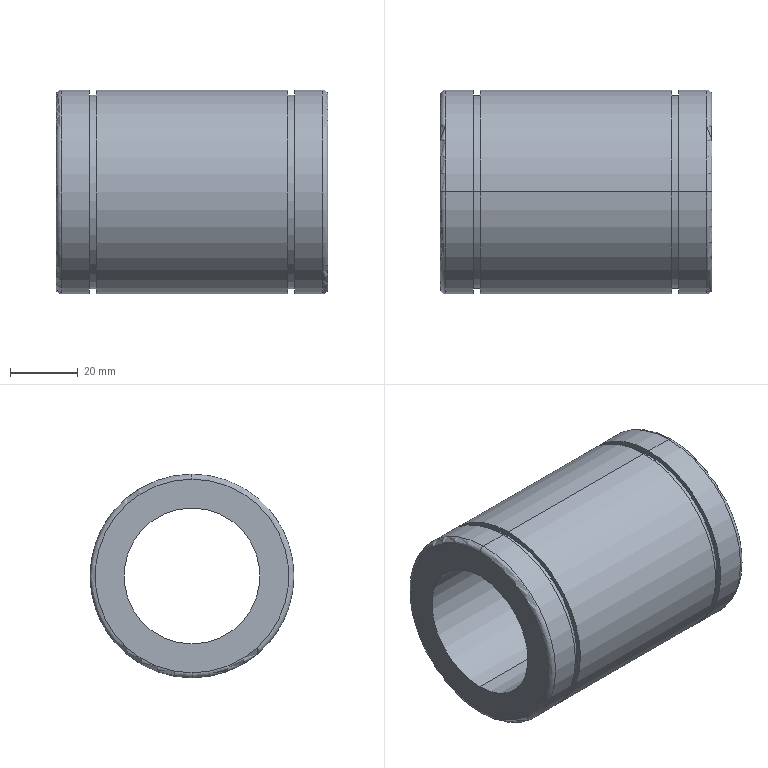Part | STEP file | LMUM40G linear bearing | 1 solid | 22 faces | box 80 x 60 x 60 mm | volume 124326 mm3 | cylinder 12 | plane 6 | torus 4 | commonest cylinder face diameters 60 x6 57 x4 40 x2
STEP:
#1=CARTESIAN_POINT('',(0.,0.,0.));
#2=DIRECTION('',(0.,0.,1.));
#3=DIRECTION('',(1.,0.,0.));
#4=AXIS2_PLACEMENT_3D('',#1,#2,#3);
#5=CARTESIAN_POINT('',(11.85,0.,-30.));
#6=VERTEX_POINT('',#5);
#7=CARTESIAN_POINT('',(11.85,0.,30.));
#8=VERTEX_POINT('',#7);
#9=CARTESIAN_POINT('',(11.85,0.,0.));
#10=DIRECTION('',(1.,0.,0.));
#11=DIRECTION('',(0.,0.,-1.));
#12=AXIS2_PLACEMENT_3D('',#9,#10,#11);
#13=CIRCLE('',#12,30.);
#14=CARTESIAN_POINT('',(80.,0.,0.));
#15=DIRECTION('',(1.,0.,0.));
#16=DIRECTION('',(0.,0.,-1.));
#17=AXIS2_PLACEMENT_3D('',#14,#15,#16);
#18=CYLINDRICAL_SURFACE('',#17,30.);
#19=CARTESIAN_POINT('',(0.,-68.15));
#20=DIRECTION('',(1.,0.));
#21=VECTOR('',#20,1.);
#22=LINE('',#19,#21);
#23=(GEOMETRIC_REPRESENTATION_CONTEXT(2)PARAMETRIC_REPRESENTATION_CONTEXT()REPRESENTATION_CONTEXT('',''));
#24=DEFINITIONAL_REPRESENTATION('',(#22),#23);
#25=PCURVE('',#18,#24);
#26=CARTESIAN_POINT('',(11.85,30.,0.));
#27=DIRECTION('',(-1.,0.,0.));
#28=DIRECTION('',(0.,0.,1.));
#29=AXIS2_PLACEMENT_3D('',#26,#27,#28);
#30=PLANE('',#29);
#31=CARTESIAN_POINT('',(-30.,-30.));
#32=CARTESIAN_POINT('',(-30.,21.962));
#33=CARTESIAN_POINT('',(15.,-4.019));
#34=CARTESIAN_POINT('',(60.,-30.));
#35=CARTESIAN_POINT('',(15.,-55.981));
#36=CARTESIAN_POINT('',(-30.,-81.962));
#37=CARTESIAN_POINT('',(-30.,-30.));
#38=(BOUNDED_CURVE()B_SPLINE_CURVE(2,(#31,#32,#33,#34,#35,#36,#37),.UNSPECIFIED.,.T.,.F.)B_SPLINE_CURVE_WITH_KNOTS((1,2,2,2,2,1),(-2.094,0.,2.094,4.189,6.283,8.378),.UNSPECIFIED.)CURVE()GEOMETRIC_REPRESENTATION_ITEM()RATIONAL_B_SPLINE_CURVE((1.,0.5,1.,0.5,1.,0.5,1.))REPRESENTATION_ITEM(''));
#39=(GEOMETRIC_REPRESENTATION_CONTEXT(2)PARAMETRIC_REPRESENTATION_CONTEXT()REPRESENTATION_CONTEXT('',''));
#40=DEFINITIONAL_REPRESENTATION('',(#38),#39);
#41=PCURVE('',#30,#40);
#42=SURFACE_CURVE('',#13,(#25,#41),.PCURVE_S1.);
#43=EDGE_CURVE('',#6,#8,#42,.T.);
#44=ORIENTED_EDGE('',*,*,#43,.T.);
#45=CARTESIAN_POINT('',(68.15,0.,30.));
#46=VERTEX_POINT('',#45);
#47=CARTESIAN_POINT('',(80.,0.,30.));
#48=DIRECTION('',(1.,0.,0.));
#49=VECTOR('',#48,1.);
#50=LINE('',#47,#49);
#51=CARTESIAN_POINT('',(3.142,0.));
#52=DIRECTION('',(0.,1.));
#53=VECTOR('',#52,1.);
#54=LINE('',#51,#53);
#55=(GEOMETRIC_REPRESENTATION_CONTEXT(2)PARAMETRIC_REPRESENTATION_CONTEXT()REPRESENTATION_CONTEXT('',''));
#56=DEFINITIONAL_REPRESENTATION('',(#54),#55);
#57=PCURVE('',#18,#56);
#58=CARTESIAN_POINT('',(80.,0.,0.));
#59=DIRECTION('',(1.,0.,0.));
#60=DIRECTION('',(0.,0.,-1.));
#61=AXIS2_PLACEMENT_3D('',#58,#59,#60);
#62=CYLINDRICAL_SURFACE('',#61,30.);
#63=CARTESIAN_POINT('',(3.142,0.));
#64=DIRECTION('',(0.,1.));
#65=VECTOR('',#64,1.);
#66=LINE('',#63,#65);
#67=(GEOMETRIC_REPRESENTATION_CONTEXT(2)PARAMETRIC_REPRESENTATION_CONTEXT()REPRESENTATION_CONTEXT('',''));
#68=DEFINITIONAL_REPRESENTATION('',(#66),#67);
#69=PCURVE('',#62,#68);
#70=SURFACE_CURVE('',#50,(#57,#69),.PCURVE_S1.);
#71=EDGE_CURVE('',#8,#46,#70,.T.);
#72=ORIENTED_EDGE('',*,*,#71,.T.);
#73=CARTESIAN_POINT('',(68.15,0.,-30.));
#74=VERTEX_POINT('',#73);
#75=CARTESIAN_POINT('',(68.15,0.,0.));
#76=DIRECTION('',(1.,0.,0.));
#77=DIRECTION('',(0.,0.,-1.));
#78=AXIS2_PLACEMENT_3D('',#75,#76,#77);
#79=CIRCLE('',#78,30.);
#80=CARTESIAN_POINT('',(0.,-11.85));
#81=DIRECTION('',(1.,0.));
#82=VECTOR('',#81,1.);
#83=LINE('',#80,#82);
#84=(GEOMETRIC_REPRESENTATION_CONTEXT(2)PARAMETRIC_REPRESENTATION_CONTEXT()REPRESENTATION_CONTEXT('',''));
#85=DEFINITIONAL_REPRESENTATION('',(#83),#84);
#86=PCURVE('',#18,#85);
#87=CARTESIAN_POINT('',(68.15,28.5,0.));
#88=DIRECTION('',(1.,0.,0.));
#89=DIRECTION('',(0.,0.,-1.));
#90=AXIS2_PLACEMENT_3D('',#87,#88,#89);
#91=PLANE('',#90);
#92=CARTESIAN_POINT('',(0.,-28.5));
#93=DIRECTION('',(1.,0.));
#94=AXIS2_PLACEMENT_2D('',#92,#93);
#95=CIRCLE('',#94,30.);
#96=(GEOMETRIC_REPRESENTATION_CONTEXT(2)PARAMETRIC_REPRESENTATION_CONTEXT()REPRESENTATION_CONTEXT('',''));
#97=DEFINITIONAL_REPRESENTATION('',(#95),#96);
#98=PCURVE('',#91,#97);
#99=SURFACE_CURVE('',#79,(#86,#98),.PCURVE_S1.);
#100=EDGE_CURVE('',#74,#46,#99,.T.);
#101=ORIENTED_EDGE('',*,*,#100,.F.);
#102=CARTESIAN_POINT('',(80.,0.,-30.));
#103=DIRECTION('',(1.,0.,0.));
#104=VECTOR('',#103,1.);
#105=LINE('',#102,#104);
#106=CARTESIAN_POINT('',(0.,0.));
#107=DIRECTION('',(0.,1.));
#108=VECTOR('',#107,1.);
#109=LINE('',#106,#108);
#110=(GEOMETRIC_REPRESENTATION_CONTEXT(2)PARAMETRIC_REPRESENTATION_CONTEXT()REPRESENTATION_CONTEXT('',''));
#111=DEFINITIONAL_REPRESENTATION('',(#109),#110);
#112=PCURVE('',#18,#111);
#113=CARTESIAN_POINT('',(6.283,0.));
#114=DIRECTION('',(0.,1.));
#115=VECTOR('',#114,1.);
#116=LINE('',#113,#115);
#117=(GEOMETRIC_REPRESENTATION_CONTEXT(2)PARAMETRIC_REPRESENTATION_CONTEXT()REPRESENTATION_CONTEXT('',''));
#118=DEFINITIONAL_REPRESENTATION('',(#116),#117);
#119=PCURVE('',#62,#118);
#120=SURFACE_CURVE('',#105,(#112,#119),.PCURVE_S1.);
#121=EDGE_CURVE('',#6,#74,#120,.T.);
#122=ORIENTED_EDGE('',*,*,#121,.F.);
#123=EDGE_LOOP('',(#44,#72,#101,#122));
#124=FACE_BOUND('',#123,.T.);
#125=ADVANCED_FACE('',(#124),#18,.T.);
#126=CARTESIAN_POINT('',(68.15,0.,-28.5));
#127=VERTEX_POINT('',#126);
#128=CARTESIAN_POINT('',(68.15,0.,28.5));
#129=VERTEX_POINT('',#128);
#130=CARTESIAN_POINT('',(68.15,0.,0.));
#131=DIRECTION('',(1.,0.,0.));
#132=DIRECTION('',(0.,0.,-1.));
#133=AXIS2_PLACEMENT_3D('',#130,#131,#132);
#134=CIRCLE('',#133,28.5);
#135=CARTESIAN_POINT('',(80.,0.,0.));
#136=DIRECTION('',(1.,0.,0.));
#137=DIRECTION('',(0.,0.,-1.));
#138=AXIS2_PLACEMENT_3D('',#135,#136,#137);
#139=CYLINDRICAL_SURFACE('',#138,28.5);
#140=CARTESIAN_POINT('',(0.,-11.85));
#141=DIRECTION('',(1.,0.));
#142=VECTOR('',#141,1.);
#143=LINE('',#140,#142);
#144=(GEOMETRIC_REPRESENTATION_CONTEXT(2)PARAMETRIC_REPRESENTATION_CONTEXT()REPRESENTATION_CONTEXT('',''));
#145=DEFINITIONAL_REPRESENTATION('',(#143),#144);
#146=PCURVE('',#139,#145);
#147=CARTESIAN_POINT('',(0.,-28.5));
#148=DIRECTION('',(1.,0.));
#149=AXIS2_PLACEMENT_2D('',#147,#148);
#150=CIRCLE('',#149,28.5);
#151=(GEOMETRIC_REPRESENTATION_CONTEXT(2)PARAMETRIC_REPRESENTATION_CONTEXT()REPRESENTATION_CONTEXT('',''));
#152=DEFINITIONAL_REPRESENTATION('',(#150),#151);
#153=PCURVE('',#91,#152);
#154=SURFACE_CURVE('',#134,(#146,#153),.PCURVE_S1.);
#155=EDGE_CURVE('',#127,#129,#154,.T.);
#156=ORIENTED_EDGE('',*,*,#155,.T.);
#157=CARTESIAN_POINT('',(70.25,0.,28.5));
#158=VERTEX_POINT('',#157);
#159=CARTESIAN_POINT('',(80.,0.,28.5));
#160=DIRECTION('',(1.,0.,0.));
#161=VECTOR('',#160,1.);
#162=LINE('',#159,#161);
#163=CARTESIAN_POINT('',(3.142,0.));
#164=DIRECTION('',(0.,1.));
#165=VECTOR('',#164,1.);
#166=LINE('',#163,#165);
#167=(GEOMETRIC_REPRESENTATION_CONTEXT(2)PARAMETRIC_REPRESENTATION_CONTEXT()REPRESENTATION_CONTEXT('',''));
#168=DEFINITIONAL_REPRESENTATION('',(#166),#167);
#169=PCURVE('',#139,#168);
#170=CARTESIAN_POINT('',(80.,0.,0.));
#171=DIRECTION('',(1.,0.,0.));
#172=DIRECTION('',(0.,0.,-1.));
#173=AXIS2_PLACEMENT_3D('',#170,#171,#172);
#174=CYLINDRICAL_SURFACE('',#173,28.5);
#175=CARTESIAN_POINT('',(3.142,0.));
#176=DIRECTION('',(0.,1.));
#177=VECTOR('',#176,1.);
#178=LINE('',#175,#177);
#179=(GEOMETRIC_REPRESENTATION_CONTEXT(2)PARAMETRIC_REPRESENTATION_CONTEXT()REPRESENTATION_CONTEXT('',''));
#180=DEFINITIONAL_REPRESENTATION('',(#178),#179);
#181=PCURVE('',#174,#180);
#182=SURFACE_CURVE('',#162,(#169,#181),.PCURVE_S1.);
#183=EDGE_CURVE('',#129,#158,#182,.T.);
#184=ORIENTED_EDGE('',*,*,#183,.T.);
#185=CARTESIAN_POINT('',(70.25,0.,-28.5));
#186=VERTEX_POINT('',#185);
#187=CARTESIAN_POINT('',(70.25,0.,0.));
#188=DIRECTION('',(1.,0.,0.));
#189=DIRECTION('',(0.,0.,-1.));
#190=AXIS2_PLACEMENT_3D('',#187,#188,#189);
#191=CIRCLE('',#190,28.5);
#192=CARTESIAN_POINT('',(0.,-9.75));
#193=DIRECTION('',(1.,0.));
#194=VECTOR('',#193,1.);
#195=LINE('',#192,#194);
#196=(GEOMETRIC_REPRESENTATION_CONTEXT(2)PARAMETRIC_REPRESENTATION_CONTEXT()REPRESENTATION_CONTEXT('',''));
#197=DEFINITIONAL_REPRESENTATION('',(#195),#196);
#198=PCURVE('',#139,#197);
#199=CARTESIAN_POINT('',(70.25,30.,0.));
#200=DIRECTION('',(-1.,0.,0.));
#201=DIRECTION('',(0.,0.,1.));
#202=AXIS2_PLACEMENT_3D('',#199,#200,#201);
#203=PLANE('',#202);
#204=CARTESIAN_POINT('',(-28.5,-30.));
#205=CARTESIAN_POINT('',(-28.5,19.363));
#206=CARTESIAN_POINT('',(14.25,-5.318));
#207=CARTESIAN_POINT('',(57.,-30.));
#208=CARTESIAN_POINT('',(14.25,-54.682));
#209=CARTESIAN_POINT('',(-28.5,-79.363));
#210=CARTESIAN_POINT('',(-28.5,-30.));
#211=(BOUNDED_CURVE()B_SPLINE_CURVE(2,(#204,#205,#206,#207,#208,#209,#210),.UNSPECIFIED.,.T.,.F.)B_SPLINE_CURVE_WITH_KNOTS((1,2,2,2,2,1),(-2.094,0.,2.094,4.189,6.283,8.378),.UNSPECIFIED.)CURVE()GEOMETRIC_REPRESENTATION_ITEM()RATIONAL_B_SPLINE_CURVE((1.,0.5,1.,0.5,1.,0.5,1.))REPRESENTATION_ITEM(''));
#212=(GEOMETRIC_REPRESENTATION_CONTEXT(2)PARAMETRIC_REPRESENTATION_CONTEXT()REPRESENTATION_CONTEXT('',''));
#213=DEFINITIONAL_REPRESENTATION('',(#211),#212);
#214=PCURVE('',#203,#213);
#215=SURFACE_CURVE('',#191,(#198,#214),.PCURVE_S1.);
#216=EDGE_CURVE('',#186,#158,#215,.T.);
#217=ORIENTED_EDGE('',*,*,#216,.F.);
#218=CARTESIAN_POINT('',(80.,0.,-28.5));
#219=DIRECTION('',(1.,0.,0.));
#220=VECTOR('',#219,1.);
#221=LINE('',#218,#220);
#222=CARTESIAN_POINT('',(0.,0.));
#223=DIRECTION('',(0.,1.));
#224=VECTOR('',#223,1.);
#225=LINE('',#222,#224);
#226=(GEOMETRIC_REPRESENTATION_CONTEXT(2)PARAMETRIC_REPRESENTATION_CONTEXT()REPRESENTATION_CONTEXT('',''));
#227=DEFINITIONAL_REPRESENTATION('',(#225),#226);
#228=PCURVE('',#139,#227);
#229=CARTESIAN_POINT('',(6.283,0.));
#230=DIRECTION('',(0.,1.));
#231=VECTOR('',#230,1.);
#232=LINE('',#229,#231);
#233=(GEOMETRIC_REPRESENTATION_CONTEXT(2)PARAMETRIC_REPRESENTATION_CONTEXT()REPRESENTATION_CONTEXT('',''));
#234=DEFINITIONAL_REPRESENTATION('',(#232),#233);
#235=PCURVE('',#174,#234);
#236=SURFACE_CURVE('',#221,(#228,#235),.PCURVE_S1.);
#237=EDGE_CURVE('',#127,#186,#236,.T.);
#238=ORIENTED_EDGE('',*,*,#237,.F.);
#239=EDGE_LOOP('',(#156,#184,#217,#238));
#240=FACE_BOUND('',#239,.T.);
#241=ADVANCED_FACE('',(#240),#139,.T.);
#242=CARTESIAN_POINT('',(9.75,0.,-28.5));
#243=VERTEX_POINT('',#242);
#244=CARTESIAN_POINT('',(9.75,0.,28.5));
#245=VERTEX_POINT('',#244);
#246=CARTESIAN_POINT('',(9.75,0.,0.));
#247=DIRECTION('',(1.,0.,0.));
#248=DIRECTION('',(0.,0.,-1.));
#249=AXIS2_PLACEMENT_3D('',#246,#247,#248);
#250=CIRCLE('',#249,28.5);
#251=CARTESIAN_POINT('',(80.,0.,0.));
#252=DIRECTION('',(1.,0.,0.));
#253=DIRECTION('',(0.,0.,-1.));
#254=AXIS2_PLACEMENT_3D('',#251,#252,#253);
#255=CYLINDRICAL_SURFACE('',#254,28.5);
#256=CARTESIAN_POINT('',(0.,-70.25));
#257=DIRECTION('',(1.,0.));
#258=VECTOR('',#257,1.);
#259=LINE('',#256,#258);
#260=(GEOMETRIC_REPRESENTATION_CONTEXT(2)PARAMETRIC_REPRESENTATION_CONTEXT()REPRESENTATION_CONTEXT('',''));
#261=DEFINITIONAL_REPRESENTATION('',(#259),#260);
#262=PCURVE('',#255,#261);
#263=CARTESIAN_POINT('',(9.75,28.5,0.));
#264=DIRECTION('',(1.,0.,0.));
#265=DIRECTION('',(0.,0.,-1.));
#266=AXIS2_PLACEMENT_3D('',#263,#264,#265);
#267=PLANE('',#266);
#268=CARTESIAN_POINT('',(0.,-28.5));
#269=DIRECTION('',(1.,0.));
#270=AXIS2_PLACEMENT_2D('',#268,#269);
#271=CIRCLE('',#270,28.5);
#272=(GEOMETRIC_REPRESENTATION_CONTEXT(2)PARAMETRIC_REPRESENTATION_CONTEXT()REPRESENTATION_CONTEXT('',''));
#273=DEFINITIONAL_REPRESENTATION('',(#271),#272);
#274=PCURVE('',#267,#273);
#275=SURFACE_CURVE('',#250,(#262,#274),.PCURVE_S1.);
#276=EDGE_CURVE('',#243,#245,#275,.T.);
#277=ORIENTED_EDGE('',*,*,#276,.T.);
#278=CARTESIAN_POINT('',(11.85,0.,28.5));
#279=VERTEX_POINT('',#278);
#280=CARTESIAN_POINT('',(80.,0.,28.5));
#281=DIRECTION('',(1.,0.,0.));
#282=VECTOR('',#281,1.);
#283=LINE('',#280,#282);
#284=CARTESIAN_POINT('',(3.142,0.));
#285=DIRECTION('',(0.,1.));
#286=VECTOR('',#285,1.);
#287=LINE('',#284,#286);
#288=(GEOMETRIC_REPRESENTATION_CONTEXT(2)PARAMETRIC_REPRESENTATION_CONTEXT()REPRESENTATION_CONTEXT('',''));
#289=DEFINITIONAL_REPRESENTATION('',(#287),#288);
#290=PCURVE('',#255,#289);
#291=CARTESIAN_POINT('',(80.,0.,0.));
#292=DIRECTION('',(1.,0.,0.));
#293=DIRECTION('',(0.,0.,-1.));
#294=AXIS2_PLACEMENT_3D('',#291,#292,#293);
#295=CYLINDRICAL_SURFACE('',#294,28.5);
#296=CARTESIAN_POINT('',(3.142,0.));
#297=DIRECTION('',(0.,1.));
#298=VECTOR('',#297,1.);
#299=LINE('',#296,#298);
#300=(GEOMETRIC_REPRESENTATION_CONTEXT(2)PARAMETRIC_REPRESENTATION_CONTEXT()REPRESENTATION_CONTEXT('',''));
#301=DEFINITIONAL_REPRESENTATION('',(#299),#300);
#302=PCURVE('',#295,#301);
#303=SURFACE_CURVE('',#283,(#290,#302),.PCURVE_S1.);
#304=EDGE_CURVE('',#245,#279,#303,.T.);
#305=ORIENTED_EDGE('',*,*,#304,.T.);
#306=CARTESIAN_POINT('',(11.85,0.,-28.5));
#307=VERTEX_POINT('',#306);
#308=CARTESIAN_POINT('',(11.85,0.,0.));
#309=DIRECTION('',(1.,0.,0.));
#310=DIRECTION('',(0.,0.,-1.));
#311=AXIS2_PLACEMENT_3D('',#308,#309,#310);
#312=CIRCLE('',#311,28.5);
#313=CARTESIAN_POINT('',(0.,-68.15));
#314=DIRECTION('',(1.,0.));
#315=VECTOR('',#314,1.);
#316=LINE('',#313,#315);
#317=(GEOMETRIC_REPRESENTATION_CONTEXT(2)PARAMETRIC_REPRESENTATION_CONTEXT()REPRESENTATION_CONTEXT('',''));
#318=DEFINITIONAL_REPRESENTATION('',(#316),#317);
#319=PCURVE('',#255,#318);
#320=CARTESIAN_POINT('',(-28.5,-30.));
#321=CARTESIAN_POINT('',(-28.5,19.363));
#322=CARTESIAN_POINT('',(14.25,-5.318));
#323=CARTESIAN_POINT('',(57.,-30.));
#324=CARTESIAN_POINT('',(14.25,-54.682));
#325=CARTESIAN_POINT('',(-28.5,-79.363));
#326=CARTESIAN_POINT('',(-28.5,-30.));
#327=(BOUNDED_CURVE()B_SPLINE_CURVE(2,(#320,#321,#322,#323,#324,#325,#326),.UNSPECIFIED.,.T.,.F.)B_SPLINE_CURVE_WITH_KNOTS((1,2,2,2,2,1),(-2.094,0.,2.094,4.189,6.283,8.378),.UNSPECIFIED.)CURVE()GEOMETRIC_REPRESENTATION_ITEM()RATIONAL_B_SPLINE_CURVE((1.,0.5,1.,0.5,1.,0.5,1.))REPRESENTATION_ITEM(''));
#328=(GEOMETRIC_REPRESENTATION_CONTEXT(2)PARAMETRIC_REPRESENTATION_CONTEXT()REPRESENTATION_CONTEXT('',''));
#329=DEFINITIONAL_REPRESENTATION('',(#327),#328);
#330=PCURVE('',#30,#329);
#331=SURFACE_CURVE('',#312,(#319,#330),.PCURVE_S1.);
#332=EDGE_CURVE('',#307,#279,#331,.T.);
#333=ORIENTED_EDGE('',*,*,#332,.F.);
#334=CARTESIAN_POINT('',(80.,0.,-28.5));
#335=DIRECTION('',(1.,0.,0.));
#336=VECTOR('',#335,1.);
#337=LINE('',#334,#336);
#338=CARTESIAN_POINT('',(0.,0.));
#339=DIRECTION('',(0.,1.));
#340=VECTOR('',#339,1.);
#341=LINE('',#338,#340);
#342=(GEOMETRIC_REPRESENTATION_CONTEXT(2)PARAMETRIC_REPRESENTATION_CONTEXT()REPRESENTATION_CONTEXT('',''));
#343=DEFINITIONAL_REPRESENTATION('',(#341),#342);
#344=PCURVE('',#255,#343);
#345=CARTESIAN_POINT('',(6.283,0.));
#346=DIRECTION('',(0.,1.));
#347=VECTOR('',#346,1.);
#348=LINE('',#345,#347);
#349=(GEOMETRIC_REPRESENTATION_CONTEXT(2)PARAMETRIC_REPRESENTATION_CONTEXT()REPRESENTATION_CONTEXT('',''));
#350=DEFINITIONAL_REPRESENTATION('',(#348),#349);
#351=PCURVE('',#295,#350);
#352=SURFACE_CURVE('',#337,(#344,#351),.PCURVE_S1.);
#353=EDGE_CURVE('',#243,#307,#352,.T.);
#354=ORIENTED_EDGE('',*,*,#353,.F.);
#355=EDGE_LOOP('',(#277,#305,#333,#354));
#356=FACE_BOUND('',#355,.T.);
#357=ADVANCED_FACE('',(#356),#255,.T.);
#358=CARTESIAN_POINT('',(70.25,0.,-30.));
#359=VERTEX_POINT('',#358);
#360=CARTESIAN_POINT('',(70.25,0.,30.));
#361=VERTEX_POINT('',#360);
#362=CARTESIAN_POINT('',(70.25,0.,0.));
#363=DIRECTION('',(1.,0.,0.));
#364=DIRECTION('',(0.,0.,-1.));
#365=AXIS2_PLACEMENT_3D('',#362,#363,#364);
#366=CIRCLE('',#365,30.);
#367=CARTESIAN_POINT('',(80.,0.,0.));
#368=DIRECTION('',(1.,0.,0.));
#369=DIRECTION('',(0.,0.,-1.));
#370=AXIS2_PLACEMENT_3D('',#367,#368,#369);
#371=CYLINDRICAL_SURFACE('',#370,30.);
#372=CARTESIAN_POINT('',(0.,-9.75));
#373=DIRECTION('',(1.,0.));
#374=VECTOR('',#373,1.);
#375=LINE('',#372,#374);
#376=(GEOMETRIC_REPRESENTATION_CONTEXT(2)PARAMETRIC_REPRESENTATION_CONTEXT()REPRESENTATION_CONTEXT('',''));
#377=DEFINITIONAL_REPRESENTATION('',(#375),#376);
#378=PCURVE('',#371,#377);
#379=CARTESIAN_POINT('',(-30.,-30.));
#380=CARTESIAN_POINT('',(-30.,21.962));
#381=CARTESIAN_POINT('',(15.,-4.019));
#382=CARTESIAN_POINT('',(60.,-30.));
#383=CARTESIAN_POINT('',(15.,-55.981));
#384=CARTESIAN_POINT('',(-30.,-81.962));
#385=CARTESIAN_POINT('',(-30.,-30.));
#386=(BOUNDED_CURVE()B_SPLINE_CURVE(2,(#379,#380,#381,#382,#383,#384,#385),.UNSPECIFIED.,.T.,.F.)B_SPLINE_CURVE_WITH_KNOTS((1,2,2,2,2,1),(-2.094,0.,2.094,4.189,6.283,8.378),.UNSPECIFIED.)CURVE()GEOMETRIC_REPRESENTATION_ITEM()RATIONAL_B_SPLINE_CURVE((1.,0.5,1.,0.5,1.,0.5,1.))REPRESENTATION_ITEM(''));
#387=(GEOMETRIC_REPRESENTATION_CONTEXT(2)PARAMETRIC_REPRESENTATION_CONTEXT()REPRESENTATION_CONTEXT('',''));
#388=DEFINITIONAL_REPRESENTATION('',(#386),#387);
#389=PCURVE('',#203,#388);
#390=SURFACE_CURVE('',#366,(#378,#389),.PCURVE_S1.);
#391=EDGE_CURVE('',#359,#361,#390,.T.);
#392=ORIENTED_EDGE('',*,*,#391,.T.);
#393=CARTESIAN_POINT('',(78.5,0.,30.));
#394=VERTEX_POINT('',#393);
#395=CARTESIAN_POINT('',(80.,0.,30.));
#396=DIRECTION('',(1.,0.,0.));
#397=VECTOR('',#396,1.);
#398=LINE('',#395,#397);
#399=CARTESIAN_POINT('',(3.142,0.));
#400=DIRECTION('',(0.,1.));
#401=VECTOR('',#400,1.);
#402=LINE('',#399,#401);
#403=(GEOMETRIC_REPRESENTATION_CONTEXT(2)PARAMETRIC_REPRESENTATION_CONTEXT()REPRESENTATION_CONTEXT('',''));
#404=DEFINITIONAL_REPRESENTATION('',(#402),#403);
#405=PCURVE('',#371,#404);
#406=CARTESIAN_POINT('',(80.,0.,0.));
#407=DIRECTION('',(1.,0.,0.));
#408=DIRECTION('',(0.,0.,-1.));
#409=AXIS2_PLACEMENT_3D('',#406,#407,#408);
#410=CYLINDRICAL_SURFACE('',#409,30.);
#411=CARTESIAN_POINT('',(3.142,0.));
#412=DIRECTION('',(0.,1.));
#413=VECTOR('',#412,1.);
#414=LINE('',#411,#413);
#415=(GEOMETRIC_REPRESENTATION_CONTEXT(2)PARAMETRIC_REPRESENTATION_CONTEXT()REPRESENTATION_CONTEXT('',''));
#416=DEFINITIONAL_REPRESENTATION('',(#414),#415);
#417=PCURVE('',#410,#416);
#418=SURFACE_CURVE('',#398,(#405,#417),.PCURVE_S1.);
#419=EDGE_CURVE('',#361,#394,#418,.T.);
#420=ORIENTED_EDGE('',*,*,#419,.T.);
#421=CARTESIAN_POINT('',(78.5,0.,-30.));
#422=VERTEX_POINT('',#421);
#423=CARTESIAN_POINT('',(78.5,0.,0.));
#424=DIRECTION('',(1.,0.,0.));
#425=DIRECTION('',(0.,0.,-1.));
#426=AXIS2_PLACEMENT_3D('',#423,#424,#425);
#427=CIRCLE('',#426,30.);
#428=CARTESIAN_POINT('',(0.,-1.5));
#429=DIRECTION('',(1.,0.));
#430=VECTOR('',#429,1.);
#431=LINE('',#428,#430);
#432=(GEOMETRIC_REPRESENTATION_CONTEXT(2)PARAMETRIC_REPRESENTATION_CONTEXT()REPRESENTATION_CONTEXT('',''));
#433=DEFINITIONAL_REPRESENTATION('',(#431),#432);
#434=PCURVE('',#371,#433);
#435=CARTESIAN_POINT('',(78.5,0.,0.));
#436=DIRECTION('',(1.,0.,0.));
#437=DIRECTION('',(0.,0.,-1.));
#438=AXIS2_PLACEMENT_3D('',#435,#436,#437);
#439=TOROIDAL_SURFACE('',#438,28.5,1.5);
#440=CARTESIAN_POINT('',(0.,0.));
#441=DIRECTION('',(1.,0.));
#442=VECTOR('',#441,1.);
#443=LINE('',#440,#442);
#444=(GEOMETRIC_REPRESENTATION_CONTEXT(2)PARAMETRIC_REPRESENTATION_CONTEXT()REPRESENTATION_CONTEXT('',''));
#445=DEFINITIONAL_REPRESENTATION('',(#443),#444);
#446=PCURVE('',#439,#445);
#447=SURFACE_CURVE('',#427,(#434,#446),.PCURVE_S1.);
#448=EDGE_CURVE('',#422,#394,#447,.T.);
#449=ORIENTED_EDGE('',*,*,#448,.F.);
#450=CARTESIAN_POINT('',(80.,0.,-30.));
#451=DIRECTION('',(1.,0.,0.));
#452=VECTOR('',#451,1.);
#453=LINE('',#450,#452);
#454=CARTESIAN_POINT('',(0.,0.));
#455=DIRECTION('',(0.,1.));
#456=VECTOR('',#455,1.);
#457=LINE('',#454,#456);
#458=(GEOMETRIC_REPRESENTATION_CONTEXT(2)PARAMETRIC_REPRESENTATION_CONTEXT()REPRESENTATION_CONTEXT('',''));
#459=DEFINITIONAL_REPRESENTATION('',(#457),#458);
#460=PCURVE('',#371,#459);
#461=CARTESIAN_POINT('',(6.283,0.));
#462=DIRECTION('',(0.,1.));
#463=VECTOR('',#462,1.);
#464=LINE('',#461,#463);
#465=(GEOMETRIC_REPRESENTATION_CONTEXT(2)PARAMETRIC_REPRESENTATION_CONTEXT()REPRESENTATION_CONTEXT('',''));
#466=DEFINITIONAL_REPRESENTATION('',(#464),#465);
#467=PCURVE('',#410,#466);
#468=SURFACE_CURVE('',#453,(#460,#467),.PCURVE_S1.);
#469=EDGE_CURVE('',#359,#422,#468,.T.);
#470=ORIENTED_EDGE('',*,*,#469,.F.);
#471=EDGE_LOOP('',(#392,#420,#449,#470));
#472=FACE_BOUND('',#471,.T.);
#473=ADVANCED_FACE('',(#472),#371,.T.);
#474=ORIENTED_EDGE('',*,*,#448,.T.);
#475=CARTESIAN_POINT('',(80.,0.,28.5));
#476=VERTEX_POINT('',#475);
#477=CARTESIAN_POINT('',(78.5,0.,28.5));
#478=DIRECTION('',(0.,1.,0.));
#479=DIRECTION('',(0.,0.,1.));
#480=AXIS2_PLACEMENT_3D('',#477,#478,#479);
#481=CIRCLE('',#480,1.5);
#482=CARTESIAN_POINT('',(3.142,0.));
#483=DIRECTION('',(0.,1.));
#484=VECTOR('',#483,1.);
#485=LINE('',#482,#484);
#486=(GEOMETRIC_REPRESENTATION_CONTEXT(2)PARAMETRIC_REPRESENTATION_CONTEXT()REPRESENTATION_CONTEXT('',''));
#487=DEFINITIONAL_REPRESENTATION('',(#485),#486);
#488=PCURVE('',#439,#487);
#489=CARTESIAN_POINT('',(78.5,0.,0.));
#490=DIRECTION('',(1.,0.,0.));
#491=DIRECTION('',(0.,0.,-1.));
#492=AXIS2_PLACEMENT_3D('',#489,#490,#491);
#493=TOROIDAL_SURFACE('',#492,28.5,1.5);
#494=CARTESIAN_POINT('',(3.142,0.));
#495=DIRECTION('',(0.,1.));
#496=VECTOR('',#495,1.);
#497=LINE('',#494,#496);
#498=(GEOMETRIC_REPRESENTATION_CONTEXT(2)PARAMETRIC_REPRESENTATION_CONTEXT()REPRESENTATION_CONTEXT('',''));
#499=DEFINITIONAL_REPRESENTATION('',(#497),#498);
#500=PCURVE('',#493,#499);
#501=SURFACE_CURVE('',#481,(#488,#500),.PCURVE_S1.);
#502=EDGE_CURVE('',#394,#476,#501,.T.);
#503=ORIENTED_EDGE('',*,*,#502,.T.);
#504=CARTESIAN_POINT('',(80.,0.,-28.5));
#505=VERTEX_POINT('',#504);
#506=CARTESIAN_POINT('',(80.,0.,0.));
#507=DIRECTION('',(1.,0.,0.));
#508=DIRECTION('',(0.,0.,-1.));
#509=AXIS2_PLACEMENT_3D('',#506,#507,#508);
#510=CIRCLE('',#509,28.5);
#511=CARTESIAN_POINT('',(0.,1.571));
#512=DIRECTION('',(1.,0.));
#513=VECTOR('',#512,1.);
#514=LINE('',#511,#513);
#515=(GEOMETRIC_REPRESENTATION_CONTEXT(2)PARAMETRIC_REPRESENTATION_CONTEXT()REPRESENTATION_CONTEXT('',''));
#516=DEFINITIONAL_REPRESENTATION('',(#514),#515);
#517=PCURVE('',#439,#516);
#518=CARTESIAN_POINT('',(80.,20.,0.));
#519=DIRECTION('',(1.,0.,0.));
#520=DIRECTION('',(0.,0.,-1.));
#521=AXIS2_PLACEMENT_3D('',#518,#519,#520);
#522=PLANE('',#521);
#523=CARTESIAN_POINT('',(0.,-20.));
#524=DIRECTION('',(1.,0.));
#525=AXIS2_PLACEMENT_2D('',#523,#524);
#526=CIRCLE('',#525,28.5);
#527=(GEOMETRIC_REPRESENTATION_CONTEXT(2)PARAMETRIC_REPRESENTATION_CONTEXT()REPRESENTATION_CONTEXT('',''));
#528=DEFINITIONAL_REPRESENTATION('',(#526),#527);
#529=PCURVE('',#522,#528);
#530=SURFACE_CURVE('',#510,(#517,#529),.PCURVE_S1.);
#531=EDGE_CURVE('',#505,#476,#530,.T.);
#532=ORIENTED_EDGE('',*,*,#531,.F.);
#533=CARTESIAN_POINT('',(78.5,0.,-28.5));
#534=DIRECTION('',(0.,-1.,0.));
#535=DIRECTION('',(0.,0.,-1.));
#536=AXIS2_PLACEMENT_3D('',#533,#534,#535);
#537=CIRCLE('',#536,1.5);
#538=CARTESIAN_POINT('',(0.,0.));
#539=DIRECTION('',(0.,1.));
#540=VECTOR('',#539,1.);
#541=LINE('',#538,#540);
#542=(GEOMETRIC_REPRESENTATION_CONTEXT(2)PARAMETRIC_REPRESENTATION_CONTEXT()REPRESENTATION_CONTEXT('',''));
#543=DEFINITIONAL_REPRESENTATION('',(#541),#542);
#544=PCURVE('',#439,#543);
#545=CARTESIAN_POINT('',(6.283,0.));
#546=DIRECTION('',(0.,1.));
#547=VECTOR('',#546,1.);
#548=LINE('',#545,#547);
#549=(GEOMETRIC_REPRESENTATION_CONTEXT(2)PARAMETRIC_REPRESENTATION_CONTEXT()REPRESENTATION_CONTEXT('',''));
#550=DEFINITIONAL_REPRESENTATION('',(#548),#549);
#551=PCURVE('',#493,#550);
#552=SURFACE_CURVE('',#537,(#544,#551),.PCURVE_S1.);
#553=EDGE_CURVE('',#422,#505,#552,.T.);
#554=ORIENTED_EDGE('',*,*,#553,.F.);
#555=EDGE_LOOP('',(#474,#503,#532,#554));
#556=FACE_BOUND('',#555,.T.);
#557=ADVANCED_FACE('',(#556),#439,.T.);
#558=CARTESIAN_POINT('',(1.5,0.,-30.));
#559=VERTEX_POINT('',#558);
#560=CARTESIAN_POINT('',(1.5,0.,30.));
#561=VERTEX_POINT('',#560);
#562=CARTESIAN_POINT('',(1.5,0.,0.));
#563=DIRECTION('',(1.,0.,0.));
#564=DIRECTION('',(0.,0.,-1.));
#565=AXIS2_PLACEMENT_3D('',#562,#563,#564);
#566=CIRCLE('',#565,30.);
#567=CARTESIAN_POINT('',(80.,0.,0.));
#568=DIRECTION('',(1.,0.,0.));
#569=DIRECTION('',(0.,0.,-1.));
#570=AXIS2_PLACEMENT_3D('',#567,#568,#569);
#571=CYLINDRICAL_SURFACE('',#570,30.);
#572=CARTESIAN_POINT('',(0.,-78.5));
#573=DIRECTION('',(1.,0.));
#574=VECTOR('',#573,1.);
#575=LINE('',#572,#574);
#576=(GEOMETRIC_REPRESENTATION_CONTEXT(2)PARAMETRIC_REPRESENTATION_CONTEXT()REPRESENTATION_CONTEXT('',''));
#577=DEFINITIONAL_REPRESENTATION('',(#575),#576);
#578=PCURVE('',#571,#577);
#579=CARTESIAN_POINT('',(1.5,0.,0.));
#580=DIRECTION('',(1.,0.,0.));
#581=DIRECTION('',(0.,0.,-1.));
#582=AXIS2_PLACEMENT_3D('',#579,#580,#581);
#583=TOROIDAL_SURFACE('',#582,28.5,1.5);
#584=CARTESIAN_POINT('',(0.,6.283));
#585=DIRECTION('',(1.,0.));
#586=VECTOR('',#585,1.);
#587=LINE('',#584,#586);
#588=(GEOMETRIC_REPRESENTATION_CONTEXT(2)PARAMETRIC_REPRESENTATION_CONTEXT()REPRESENTATION_CONTEXT('',''));
#589=DEFINITIONAL_REPRESENTATION('',(#587),#588);
#590=PCURVE('',#583,#589);
#591=SURFACE_CURVE('',#566,(#578,#590),.PCURVE_S1.);
#592=EDGE_CURVE('',#559,#561,#591,.T.);
#593=ORIENTED_EDGE('',*,*,#592,.T.);
#594=CARTESIAN_POINT('',(9.75,0.,30.));
#595=VERTEX_POINT('',#594);
#596=CARTESIAN_POINT('',(80.,0.,30.));
#597=DIRECTION('',(1.,0.,0.));
#598=VECTOR('',#597,1.);
#599=LINE('',#596,#598);
#600=CARTESIAN_POINT('',(3.142,0.));
#601=DIRECTION('',(0.,1.));
#602=VECTOR('',#601,1.);
#603=LINE('',#600,#602);
#604=(GEOMETRIC_REPRESENTATION_CONTEXT(2)PARAMETRIC_REPRESENTATION_CONTEXT()REPRESENTATION_CONTEXT('',''));
#605=DEFINITIONAL_REPRESENTATION('',(#603),#604);
#606=PCURVE('',#571,#605);
#607=CARTESIAN_POINT('',(80.,0.,0.));
#608=DIRECTION('',(1.,0.,0.));
#609=DIRECTION('',(0.,0.,-1.));
#610=AXIS2_PLACEMENT_3D('',#607,#608,#609);
#611=CYLINDRICAL_SURFACE('',#610,30.);
#612=CARTESIAN_POINT('',(3.142,0.));
#613=DIRECTION('',(0.,1.));
#614=VECTOR('',#613,1.);
#615=LINE('',#612,#614);
#616=(GEOMETRIC_REPRESENTATION_CONTEXT(2)PARAMETRIC_REPRESENTATION_CONTEXT()REPRESENTATION_CONTEXT('',''));
#617=DEFINITIONAL_REPRESENTATION('',(#615),#616);
#618=PCURVE('',#611,#617);
#619=SURFACE_CURVE('',#599,(#606,#618),.PCURVE_S1.);
#620=EDGE_CURVE('',#561,#595,#619,.T.);
#621=ORIENTED_EDGE('',*,*,#620,.T.);
#622=CARTESIAN_POINT('',(9.75,0.,-30.));
#623=VERTEX_POINT('',#622);
#624=CARTESIAN_POINT('',(9.75,0.,0.));
#625=DIRECTION('',(1.,0.,0.));
#626=DIRECTION('',(0.,0.,-1.));
#627=AXIS2_PLACEMENT_3D('',#624,#625,#626);
#628=CIRCLE('',#627,30.);
#629=CARTESIAN_POINT('',(0.,-70.25));
#630=DIRECTION('',(1.,0.));
#631=VECTOR('',#630,1.);
#632=LINE('',#629,#631);
#633=(GEOMETRIC_REPRESENTATION_CONTEXT(2)PARAMETRIC_REPRESENTATION_CONTEXT()REPRESENTATION_CONTEXT('',''));
#634=DEFINITIONAL_REPRESENTATION('',(#632),#633);
#635=PCURVE('',#571,#634);
#636=CARTESIAN_POINT('',(0.,-28.5));
#637=DIRECTION('',(1.,0.));
#638=AXIS2_PLACEMENT_2D('',#636,#637);
#639=CIRCLE('',#638,30.);
#640=(GEOMETRIC_REPRESENTATION_CONTEXT(2)PARAMETRIC_REPRESENTATION_CONTEXT()REPRESENTATION_CONTEXT('',''));
#641=DEFINITIONAL_REPRESENTATION('',(#639),#640);
#642=PCURVE('',#267,#641);
#643=SURFACE_CURVE('',#628,(#635,#642),.PCURVE_S1.);
#644=EDGE_CURVE('',#623,#595,#643,.T.);
#645=ORIENTED_EDGE('',*,*,#644,.F.);
#646=CARTESIAN_POINT('',(80.,0.,-30.));
#647=DIRECTION('',(1.,0.,0.));
#648=VECTOR('',#647,1.);
#649=LINE('',#646,#648);
#650=CARTESIAN_POINT('',(0.,0.));
#651=DIRECTION('',(0.,1.));
#652=VECTOR('',#651,1.);
#653=LINE('',#650,#652);
#654=(GEOMETRIC_REPRESENTATION_CONTEXT(2)PARAMETRIC_REPRESENTATION_CONTEXT()REPRESENTATION_CONTEXT('',''));
#655=DEFINITIONAL_REPRESENTATION('',(#653),#654);
#656=PCURVE('',#571,#655);
#657=CARTESIAN_POINT('',(6.283,0.));
#658=DIRECTION('',(0.,1.));
#659=VECTOR('',#658,1.);
#660=LINE('',#657,#659);
#661=(GEOMETRIC_REPRESENTATION_CONTEXT(2)PARAMETRIC_REPRESENTATION_CONTEXT()REPRESENTATION_CONTEXT('',''));
#662=DEFINITIONAL_REPRESENTATION('',(#660),#661);
#663=PCURVE('',#611,#662);
#664=SURFACE_CURVE('',#649,(#656,#663),.PCURVE_S1.);
#665=EDGE_CURVE('',#559,#623,#664,.T.);
#666=ORIENTED_EDGE('',*,*,#665,.F.);
#667=EDGE_LOOP('',(#593,#621,#645,#666));
#668=FACE_BOUND('',#667,.T.);
#669=ADVANCED_FACE('',(#668),#571,.T.);
#670=CARTESIAN_POINT('',(0.,0.,-28.5));
#671=VERTEX_POINT('',#670);
#672=CARTESIAN_POINT('',(0.,0.,28.5));
#673=VERTEX_POINT('',#672);
#674=CARTESIAN_POINT('',(0.,0.,0.));
#675=DIRECTION('',(1.,0.,0.));
#676=DIRECTION('',(0.,0.,-1.));
#677=AXIS2_PLACEMENT_3D('',#674,#675,#676);
#678=CIRCLE('',#677,28.5);
#679=CARTESIAN_POINT('',(0.,4.712));
#680=DIRECTION('',(1.,0.));
#681=VECTOR('',#680,1.);
#682=LINE('',#679,#681);
#683=(GEOMETRIC_REPRESENTATION_CONTEXT(2)PARAMETRIC_REPRESENTATION_CONTEXT()REPRESENTATION_CONTEXT('',''));
#684=DEFINITIONAL_REPRESENTATION('',(#682),#683);
#685=PCURVE('',#583,#684);
#686=CARTESIAN_POINT('',(0.,28.5,0.));
#687=DIRECTION('',(-1.,0.,0.));
#688=DIRECTION('',(0.,0.,1.));
#689=AXIS2_PLACEMENT_3D('',#686,#687,#688);
#690=PLANE('',#689);
#691=CARTESIAN_POINT('',(-28.5,-28.5));
#692=CARTESIAN_POINT('',(-28.5,20.863));
#693=CARTESIAN_POINT('',(14.25,-3.818));
#694=CARTESIAN_POINT('',(57.,-28.5));
#695=CARTESIAN_POINT('',(14.25,-53.182));
#696=CARTESIAN_POINT('',(-28.5,-77.863));
#697=CARTESIAN_POINT('',(-28.5,-28.5));
#698=(BOUNDED_CURVE()B_SPLINE_CURVE(2,(#691,#692,#693,#694,#695,#696,#697),.UNSPECIFIED.,.T.,.F.)B_SPLINE_CURVE_WITH_KNOTS((1,2,2,2,2,1),(-2.094,0.,2.094,4.189,6.283,8.378),.UNSPECIFIED.)CURVE()GEOMETRIC_REPRESENTATION_ITEM()RATIONAL_B_SPLINE_CURVE((1.,0.5,1.,0.5,1.,0.5,1.))REPRESENTATION_ITEM(''));
#699=(GEOMETRIC_REPRESENTATION_CONTEXT(2)PARAMETRIC_REPRESENTATION_CONTEXT()REPRESENTATION_CONTEXT('',''));
#700=DEFINITIONAL_REPRESENTATION('',(#698),#699);
#701=PCURVE('',#690,#700);
#702=SURFACE_CURVE('',#678,(#685,#701),.PCURVE_S1.);
#703=EDGE_CURVE('',#671,#673,#702,.T.);
#704=ORIENTED_EDGE('',*,*,#703,.T.);
#705=CARTESIAN_POINT('',(1.5,0.,28.5));
#706=DIRECTION('',(0.,1.,0.));
#707=DIRECTION('',(0.,0.,1.));
#708=AXIS2_PLACEMENT_3D('',#705,#706,#707);
#709=CIRCLE('',#708,1.5);
#710=CARTESIAN_POINT('',(3.142,0.));
#711=DIRECTION('',(0.,1.));
#712=VECTOR('',#711,1.);
#713=LINE('',#710,#712);
#714=(GEOMETRIC_REPRESENTATION_CONTEXT(2)PARAMETRIC_REPRESENTATION_CONTEXT()REPRESENTATION_CONTEXT('',''));
#715=DEFINITIONAL_REPRESENTATION('',(#713),#714);
#716=PCURVE('',#583,#715);
#717=CARTESIAN_POINT('',(1.5,0.,0.));
#718=DIRECTION('',(1.,0.,0.));
#719=DIRECTION('',(0.,0.,-1.));
#720=AXIS2_PLACEMENT_3D('',#717,#718,#719);
#721=TOROIDAL_SURFACE('',#720,28.5,1.5);
#722=CARTESIAN_POINT('',(3.142,0.));
#723=DIRECTION('',(0.,1.));
#724=VECTOR('',#723,1.);
#725=LINE('',#722,#724);
#726=(GEOMETRIC_REPRESENTATION_CONTEXT(2)PARAMETRIC_REPRESENTATION_CONTEXT()REPRESENTATION_CONTEXT('',''));
#727=DEFINITIONAL_REPRESENTATION('',(#725),#726);
#728=PCURVE('',#721,#727);
#729=SURFACE_CURVE('',#709,(#716,#728),.PCURVE_S1.);
#730=EDGE_CURVE('',#673,#561,#729,.T.);
#731=ORIENTED_EDGE('',*,*,#730,.T.);
#732=ORIENTED_EDGE('',*,*,#592,.F.);
#733=CARTESIAN_POINT('',(1.5,0.,-28.5));
#734=DIRECTION('',(0.,-1.,0.));
#735=DIRECTION('',(0.,0.,-1.));
#736=AXIS2_PLACEMENT_3D('',#733,#734,#735);
#737=CIRCLE('',#736,1.5);
#738=CARTESIAN_POINT('',(0.,0.));
#739=DIRECTION('',(0.,1.));
#740=VECTOR('',#739,1.);
#741=LINE('',#738,#740);
#742=(GEOMETRIC_REPRESENTATION_CONTEXT(2)PARAMETRIC_REPRESENTATION_CONTEXT()REPRESENTATION_CONTEXT('',''));
#743=DEFINITIONAL_REPRESENTATION('',(#741),#742);
#744=PCURVE('',#583,#743);
#745=CARTESIAN_POINT('',(6.283,0.));
#746=DIRECTION('',(0.,1.));
#747=VECTOR('',#746,1.);
#748=LINE('',#745,#747);
#749=(GEOMETRIC_REPRESENTATION_CONTEXT(2)PARAMETRIC_REPRESENTATION_CONTEXT()REPRESENTATION_CONTEXT('',''));
#750=DEFINITIONAL_REPRESENTATION('',(#748),#749);
#751=PCURVE('',#721,#750);
#752=SURFACE_CURVE('',#737,(#744,#751),.PCURVE_S1.);
#753=EDGE_CURVE('',#671,#559,#752,.T.);
#754=ORIENTED_EDGE('',*,*,#753,.F.);
#755=EDGE_LOOP('',(#704,#731,#732,#754));
#756=FACE_BOUND('',#755,.T.);
#757=ADVANCED_FACE('',(#756),#583,.T.);
#758=CARTESIAN_POINT('',(0.,0.,-20.));
#759=VERTEX_POINT('',#758);
#760=CARTESIAN_POINT('',(80.,0.,-20.));
#761=VERTEX_POINT('',#760);
#762=CARTESIAN_POINT('',(80.,0.,-20.));
#763=DIRECTION('',(1.,0.,0.));
#764=VECTOR('',#763,1.);
#765=LINE('',#762,#764);
#766=CARTESIAN_POINT('',(80.,0.,0.));
#767=DIRECTION('',(1.,0.,0.));
#768=DIRECTION('',(0.,0.,-1.));
#769=AXIS2_PLACEMENT_3D('',#766,#767,#768);
#770=CYLINDRICAL_SURFACE('',#769,20.);
#771=CARTESIAN_POINT('',(6.283,0.));
#772=DIRECTION('',(0.,1.));
#773=VECTOR('',#772,1.);
#774=LINE('',#771,#773);
#775=(GEOMETRIC_REPRESENTATION_CONTEXT(2)PARAMETRIC_REPRESENTATION_CONTEXT()REPRESENTATION_CONTEXT('',''));
#776=DEFINITIONAL_REPRESENTATION('',(#774),#775);
#777=PCURVE('',#770,#776);
#778=CARTESIAN_POINT('',(80.,0.,0.));
#779=DIRECTION('',(1.,0.,0.));
#780=DIRECTION('',(0.,0.,-1.));
#781=AXIS2_PLACEMENT_3D('',#778,#779,#780);
#782=CYLINDRICAL_SURFACE('',#781,20.);
#783=CARTESIAN_POINT('',(0.,0.));
#784=DIRECTION('',(0.,1.));
#785=VECTOR('',#784,1.);
#786=LINE('',#783,#785);
#787=(GEOMETRIC_REPRESENTATION_CONTEXT(2)PARAMETRIC_REPRESENTATION_CONTEXT()REPRESENTATION_CONTEXT('',''));
#788=DEFINITIONAL_REPRESENTATION('',(#786),#787);
#789=PCURVE('',#782,#788);
#790=SURFACE_CURVE('',#765,(#777,#789),.PCURVE_S1.);
#791=EDGE_CURVE('',#759,#761,#790,.T.);
#792=ORIENTED_EDGE('',*,*,#791,.T.);
#793=CARTESIAN_POINT('',(80.,0.,20.));
#794=VERTEX_POINT('',#793);
#795=CARTESIAN_POINT('',(80.,0.,0.));
#796=DIRECTION('',(1.,0.,0.));
#797=DIRECTION('',(0.,0.,-1.));
#798=AXIS2_PLACEMENT_3D('',#795,#796,#797);
#799=CIRCLE('',#798,20.);
#800=CARTESIAN_POINT('',(0.,0.));
#801=DIRECTION('',(1.,0.));
#802=VECTOR('',#801,1.);
#803=LINE('',#800,#802);
#804=(GEOMETRIC_REPRESENTATION_CONTEXT(2)PARAMETRIC_REPRESENTATION_CONTEXT()REPRESENTATION_CONTEXT('',''));
#805=DEFINITIONAL_REPRESENTATION('',(#803),#804);
#806=PCURVE('',#770,#805);
#807=CARTESIAN_POINT('',(0.,-20.));
#808=DIRECTION('',(1.,0.));
#809=AXIS2_PLACEMENT_2D('',#807,#808);
#810=CIRCLE('',#809,20.);
#811=(GEOMETRIC_REPRESENTATION_CONTEXT(2)PARAMETRIC_REPRESENTATION_CONTEXT()REPRESENTATION_CONTEXT('',''));
#812=DEFINITIONAL_REPRESENTATION('',(#810),#811);
#813=PCURVE('',#522,#812);
#814=SURFACE_CURVE('',#799,(#806,#813),.PCURVE_S1.);
#815=EDGE_CURVE('',#794,#761,#814,.T.);
#816=ORIENTED_EDGE('',*,*,#815,.F.);
#817=CARTESIAN_POINT('',(0.,0.,20.));
#818=VERTEX_POINT('',#817);
#819=CARTESIAN_POINT('',(80.,0.,20.));
#820=DIRECTION('',(1.,0.,0.));
#821=VECTOR('',#820,1.);
#822=LINE('',#819,#821);
#823=CARTESIAN_POINT('',(3.142,0.));
#824=DIRECTION('',(0.,1.));
#825=VECTOR('',#824,1.);
#826=LINE('',#823,#825);
#827=(GEOMETRIC_REPRESENTATION_CONTEXT(2)PARAMETRIC_REPRESENTATION_CONTEXT()REPRESENTATION_CONTEXT('',''));
#828=DEFINITIONAL_REPRESENTATION('',(#826),#827);
#829=PCURVE('',#770,#828);
#830=CARTESIAN_POINT('',(3.142,0.));
#831=DIRECTION('',(0.,1.));
#832=VECTOR('',#831,1.);
#833=LINE('',#830,#832);
#834=(GEOMETRIC_REPRESENTATION_CONTEXT(2)PARAMETRIC_REPRESENTATION_CONTEXT()REPRESENTATION_CONTEXT('',''));
#835=DEFINITIONAL_REPRESENTATION('',(#833),#834);
#836=PCURVE('',#782,#835);
#837=SURFACE_CURVE('',#822,(#829,#836),.PCURVE_S1.);
#838=EDGE_CURVE('',#818,#794,#837,.T.);
#839=ORIENTED_EDGE('',*,*,#838,.F.);
#840=CARTESIAN_POINT('',(0.,0.,0.));
#841=DIRECTION('',(1.,0.,0.));
#842=DIRECTION('',(0.,0.,-1.));
#843=AXIS2_PLACEMENT_3D('',#840,#841,#842);
#844=CIRCLE('',#843,20.);
#845=CARTESIAN_POINT('',(0.,-80.));
#846=DIRECTION('',(1.,0.));
#847=VECTOR('',#846,1.);
#848=LINE('',#845,#847);
#849=(GEOMETRIC_REPRESENTATION_CONTEXT(2)PARAMETRIC_REPRESENTATION_CONTEXT()REPRESENTATION_CONTEXT('',''));
#850=DEFINITIONAL_REPRESENTATION('',(#848),#849);
#851=PCURVE('',#770,#850);
#852=CARTESIAN_POINT('',(-20.,-28.5));
#853=CARTESIAN_POINT('',(-20.,6.141));
#854=CARTESIAN_POINT('',(10.,-11.179));
#855=CARTESIAN_POINT('',(40.,-28.5));
#856=CARTESIAN_POINT('',(10.,-45.821));
#857=CARTESIAN_POINT('',(-20.,-63.141));
#858=CARTESIAN_POINT('',(-20.,-28.5));
#859=(BOUNDED_CURVE()B_SPLINE_CURVE(2,(#852,#853,#854,#855,#856,#857,#858),.UNSPECIFIED.,.T.,.F.)B_SPLINE_CURVE_WITH_KNOTS((1,2,2,2,2,1),(-2.094,0.,2.094,4.189,6.283,8.378),.UNSPECIFIED.)CURVE()GEOMETRIC_REPRESENTATION_ITEM()RATIONAL_B_SPLINE_CURVE((1.,0.5,1.,0.5,1.,0.5,1.))REPRESENTATION_ITEM(''));
#860=(GEOMETRIC_REPRESENTATION_CONTEXT(2)PARAMETRIC_REPRESENTATION_CONTEXT()REPRESENTATION_CONTEXT('',''));
#861=DEFINITIONAL_REPRESENTATION('',(#859),#860);
#862=PCURVE('',#690,#861);
#863=SURFACE_CURVE('',#844,(#851,#862),.PCURVE_S1.);
#864=EDGE_CURVE('',#818,#759,#863,.T.);
#865=ORIENTED_EDGE('',*,*,#864,.T.);
#866=EDGE_LOOP('',(#792,#816,#839,#865));
#867=FACE_BOUND('',#866,.F.);
#868=ADVANCED_FACE('',(#867),#770,.F.);
#869=CARTESIAN_POINT('',(0.,0.,0.));
#870=DIRECTION('',(1.,0.,0.));
#871=DIRECTION('',(0.,0.,-1.));
#872=AXIS2_PLACEMENT_3D('',#869,#870,#871);
#873=CIRCLE('',#872,20.);
#874=CARTESIAN_POINT('',(-20.,-28.5));
#875=CARTESIAN_POINT('',(-20.,6.141));
#876=CARTESIAN_POINT('',(10.,-11.179));
#877=CARTESIAN_POINT('',(40.,-28.5));
#878=CARTESIAN_POINT('',(10.,-45.821));
#879=CARTESIAN_POINT('',(-20.,-63.141));
#880=CARTESIAN_POINT('',(-20.,-28.5));
#881=(BOUNDED_CURVE()B_SPLINE_CURVE(2,(#874,#875,#876,#877,#878,#879,#880),.UNSPECIFIED.,.T.,.F.)B_SPLINE_CURVE_WITH_KNOTS((1,2,2,2,2,1),(-2.094,0.,2.094,4.189,6.283,8.378),.UNSPECIFIED.)CURVE()GEOMETRIC_REPRESENTATION_ITEM()RATIONAL_B_SPLINE_CURVE((1.,0.5,1.,0.5,1.,0.5,1.))REPRESENTATION_ITEM(''));
#882=(GEOMETRIC_REPRESENTATION_CONTEXT(2)PARAMETRIC_REPRESENTATION_CONTEXT()REPRESENTATION_CONTEXT('',''));
#883=DEFINITIONAL_REPRESENTATION('',(#881),#882);
#884=PCURVE('',#690,#883);
#885=CARTESIAN_POINT('',(0.,-80.));
#886=DIRECTION('',(1.,0.));
#887=VECTOR('',#886,1.);
#888=LINE('',#885,#887);
#889=(GEOMETRIC_REPRESENTATION_CONTEXT(2)PARAMETRIC_REPRESENTATION_CONTEXT()REPRESENTATION_CONTEXT('',''));
#890=DEFINITIONAL_REPRESENTATION('',(#888),#889);
#891=PCURVE('',#782,#890);
#892=SURFACE_CURVE('',#873,(#884,#891),.PCURVE_S1.);
#893=EDGE_CURVE('',#759,#818,#892,.T.);
#894=ORIENTED_EDGE('',*,*,#893,.T.);
#895=ORIENTED_EDGE('',*,*,#864,.T.);
#896=EDGE_LOOP('',(#894,#895));
#897=FACE_BOUND('',#896,.T.);
#898=ORIENTED_EDGE('',*,*,#703,.F.);
#899=CARTESIAN_POINT('',(0.,0.,0.));
#900=DIRECTION('',(1.,0.,0.));
#901=DIRECTION('',(0.,0.,-1.));
#902=AXIS2_PLACEMENT_3D('',#899,#900,#901);
#903=CIRCLE('',#902,28.5);
#904=CARTESIAN_POINT('',(-28.5,-28.5));
#905=CARTESIAN_POINT('',(-28.5,20.863));
#906=CARTESIAN_POINT('',(14.25,-3.818));
#907=CARTESIAN_POINT('',(57.,-28.5));
#908=CARTESIAN_POINT('',(14.25,-53.182));
#909=CARTESIAN_POINT('',(-28.5,-77.863));
#910=CARTESIAN_POINT('',(-28.5,-28.5));
#911=(BOUNDED_CURVE()B_SPLINE_CURVE(2,(#904,#905,#906,#907,#908,#909,#910),.UNSPECIFIED.,.T.,.F.)B_SPLINE_CURVE_WITH_KNOTS((1,2,2,2,2,1),(-2.094,0.,2.094,4.189,6.283,8.378),.UNSPECIFIED.)CURVE()GEOMETRIC_REPRESENTATION_ITEM()RATIONAL_B_SPLINE_CURVE((1.,0.5,1.,0.5,1.,0.5,1.))REPRESENTATION_ITEM(''));
#912=(GEOMETRIC_REPRESENTATION_CONTEXT(2)PARAMETRIC_REPRESENTATION_CONTEXT()REPRESENTATION_CONTEXT('',''));
#913=DEFINITIONAL_REPRESENTATION('',(#911),#912);
#914=PCURVE('',#690,#913);
#915=CARTESIAN_POINT('',(0.,4.712));
#916=DIRECTION('',(1.,0.));
#917=VECTOR('',#916,1.);
#918=LINE('',#915,#917);
#919=(GEOMETRIC_REPRESENTATION_CONTEXT(2)PARAMETRIC_REPRESENTATION_CONTEXT()REPRESENTATION_CONTEXT('',''));
#920=DEFINITIONAL_REPRESENTATION('',(#918),#919);
#921=PCURVE('',#721,#920);
#922=SURFACE_CURVE('',#903,(#914,#921),.PCURVE_S1.);
#923=EDGE_CURVE('',#673,#671,#922,.T.);
#924=ORIENTED_EDGE('',*,*,#923,.F.);
#925=EDGE_LOOP('',(#898,#924));
#926=FACE_BOUND('',#925,.T.);
#927=ADVANCED_FACE('',(#897,#926),#690,.T.);
#928=CARTESIAN_POINT('',(80.,0.,0.));
#929=DIRECTION('',(1.,0.,0.));
#930=DIRECTION('',(0.,0.,-1.));
#931=AXIS2_PLACEMENT_3D('',#928,#929,#930);
#932=CIRCLE('',#931,20.);
#933=CARTESIAN_POINT('',(0.,0.));
#934=DIRECTION('',(1.,0.));
#935=VECTOR('',#934,1.);
#936=LINE('',#933,#935);
#937=(GEOMETRIC_REPRESENTATION_CONTEXT(2)PARAMETRIC_REPRESENTATION_CONTEXT()REPRESENTATION_CONTEXT('',''));
#938=DEFINITIONAL_REPRESENTATION('',(#936),#937);
#939=PCURVE('',#782,#938);
#940=CARTESIAN_POINT('',(0.,-20.));
#941=DIRECTION('',(1.,0.));
#942=AXIS2_PLACEMENT_2D('',#940,#941);
#943=CIRCLE('',#942,20.);
#944=(GEOMETRIC_REPRESENTATION_CONTEXT(2)PARAMETRIC_REPRESENTATION_CONTEXT()REPRESENTATION_CONTEXT('',''));
#945=DEFINITIONAL_REPRESENTATION('',(#943),#944);
#946=PCURVE('',#522,#945);
#947=SURFACE_CURVE('',#932,(#939,#946),.PCURVE_S1.);
#948=EDGE_CURVE('',#761,#794,#947,.T.);
#949=ORIENTED_EDGE('',*,*,#948,.F.);
#950=ORIENTED_EDGE('',*,*,#791,.F.);
#951=ORIENTED_EDGE('',*,*,#893,.T.);
#952=ORIENTED_EDGE('',*,*,#838,.T.);
#953=EDGE_LOOP('',(#949,#950,#951,#952));
#954=FACE_BOUND('',#953,.F.);
#955=ADVANCED_FACE('',(#954),#782,.F.);
#956=ORIENTED_EDGE('',*,*,#730,.F.);
#957=ORIENTED_EDGE('',*,*,#923,.T.);
#958=ORIENTED_EDGE('',*,*,#753,.T.);
#959=CARTESIAN_POINT('',(1.5,0.,0.));
#960=DIRECTION('',(1.,0.,0.));
#961=DIRECTION('',(0.,0.,-1.));
#962=AXIS2_PLACEMENT_3D('',#959,#960,#961);
#963=CIRCLE('',#962,30.);
#964=CARTESIAN_POINT('',(0.,6.283));
#965=DIRECTION('',(1.,0.));
#966=VECTOR('',#965,1.);
#967=LINE('',#964,#966);
#968=(GEOMETRIC_REPRESENTATION_CONTEXT(2)PARAMETRIC_REPRESENTATION_CONTEXT()REPRESENTATION_CONTEXT('',''));
#969=DEFINITIONAL_REPRESENTATION('',(#967),#968);
#970=PCURVE('',#721,#969);
#971=CARTESIAN_POINT('',(0.,-78.5));
#972=DIRECTION('',(1.,0.));
#973=VECTOR('',#972,1.);
#974=LINE('',#971,#973);
#975=(GEOMETRIC_REPRESENTATION_CONTEXT(2)PARAMETRIC_REPRESENTATION_CONTEXT()REPRESENTATION_CONTEXT('',''));
#976=DEFINITIONAL_REPRESENTATION('',(#974),#975);
#977=PCURVE('',#611,#976);
#978=SURFACE_CURVE('',#963,(#970,#977),.PCURVE_S1.);
#979=EDGE_CURVE('',#561,#559,#978,.T.);
#980=ORIENTED_EDGE('',*,*,#979,.F.);
#981=EDGE_LOOP('',(#956,#957,#958,#980));
#982=FACE_BOUND('',#981,.T.);
#983=ADVANCED_FACE('',(#982),#721,.T.);
#984=ORIENTED_EDGE('',*,*,#531,.T.);
#985=CARTESIAN_POINT('',(80.,0.,0.));
#986=DIRECTION('',(1.,0.,0.));
#987=DIRECTION('',(0.,0.,-1.));
#988=AXIS2_PLACEMENT_3D('',#985,#986,#987);
#989=CIRCLE('',#988,28.5);
#990=CARTESIAN_POINT('',(0.,-20.));
#991=DIRECTION('',(1.,0.));
#992=AXIS2_PLACEMENT_2D('',#990,#991);
#993=CIRCLE('',#992,28.5);
#994=(GEOMETRIC_REPRESENTATION_CONTEXT(2)PARAMETRIC_REPRESENTATION_CONTEXT()REPRESENTATION_CONTEXT('',''));
#995=DEFINITIONAL_REPRESENTATION('',(#993),#994);
#996=PCURVE('',#522,#995);
#997=CARTESIAN_POINT('',(0.,1.571));
#998=DIRECTION('',(1.,0.));
#999=VECTOR('',#998,1.);
#1000=LINE('',#997,#999);
#1001=(GEOMETRIC_REPRESENTATION_CONTEXT(2)PARAMETRIC_REPRESENTATION_CONTEXT()REPRESENTATION_CONTEXT('',''));
#1002=DEFINITIONAL_REPRESENTATION('',(#1000),#1001);
#1003=PCURVE('',#493,#1002);
#1004=SURFACE_CURVE('',#989,(#996,#1003),.PCURVE_S1.);
#1005=EDGE_CURVE('',#476,#505,#1004,.T.);
#1006=ORIENTED_EDGE('',*,*,#1005,.T.);
#1007=EDGE_LOOP('',(#984,#1006));
#1008=FACE_BOUND('',#1007,.T.);
#1009=ORIENTED_EDGE('',*,*,#948,.F.);
#1010=ORIENTED_EDGE('',*,*,#815,.F.);
#1011=EDGE_LOOP('',(#1009,#1010));
#1012=FACE_BOUND('',#1011,.T.);
#1013=ADVANCED_FACE('',(#1008,#1012),#522,.T.);
#1014=ORIENTED_EDGE('',*,*,#620,.F.);
#1015=ORIENTED_EDGE('',*,*,#979,.T.);
#1016=ORIENTED_EDGE('',*,*,#665,.T.);
#1017=CARTESIAN_POINT('',(9.75,0.,0.));
#1018=DIRECTION('',(1.,0.,0.));
#1019=DIRECTION('',(0.,0.,-1.));
#1020=AXIS2_PLACEMENT_3D('',#1017,#1018,#1019);
#1021=CIRCLE('',#1020,30.);
#1022=CARTESIAN_POINT('',(0.,-70.25));
#1023=DIRECTION('',(1.,0.));
#1024=VECTOR('',#1023,1.);
#1025=LINE('',#1022,#1024);
#1026=(GEOMETRIC_REPRESENTATION_CONTEXT(2)PARAMETRIC_REPRESENTATION_CONTEXT()REPRESENTATION_CONTEXT('',''));
#1027=DEFINITIONAL_REPRESENTATION('',(#1025),#1026);
#1028=PCURVE('',#611,#1027);
#1029=CARTESIAN_POINT('',(0.,-28.5));
#1030=DIRECTION('',(1.,0.));
#1031=AXIS2_PLACEMENT_2D('',#1029,#1030);
#1032=CIRCLE('',#1031,30.);
#1033=(GEOMETRIC_REPRESENTATION_CONTEXT(2)PARAMETRIC_REPRESENTATION_CONTEXT()REPRESENTATION_CONTEXT('',''));
#1034=DEFINITIONAL_REPRESENTATION('',(#1032),#1033);
#1035=PCURVE('',#267,#1034);
#1036=SURFACE_CURVE('',#1021,(#1028,#1035),.PCURVE_S1.);
#1037=EDGE_CURVE('',#595,#623,#1036,.T.);
#1038=ORIENTED_EDGE('',*,*,#1037,.F.);
#1039=EDGE_LOOP('',(#1014,#1015,#1016,#1038));
#1040=FACE_BOUND('',#1039,.T.);
#1041=ADVANCED_FACE('',(#1040),#611,.T.);
#1042=ORIENTED_EDGE('',*,*,#502,.F.);
#1043=CARTESIAN_POINT('',(78.5,0.,0.));
#1044=DIRECTION('',(1.,0.,0.));
#1045=DIRECTION('',(0.,0.,-1.));
#1046=AXIS2_PLACEMENT_3D('',#1043,#1044,#1045);
#1047=CIRCLE('',#1046,30.);
#1048=CARTESIAN_POINT('',(0.,0.));
#1049=DIRECTION('',(1.,0.));
#1050=VECTOR('',#1049,1.);
#1051=LINE('',#1048,#1050);
#1052=(GEOMETRIC_REPRESENTATION_CONTEXT(2)PARAMETRIC_REPRESENTATION_CONTEXT()REPRESENTATION_CONTEXT('',''));
#1053=DEFINITIONAL_REPRESENTATION('',(#1051),#1052);
#1054=PCURVE('',#493,#1053);
#1055=CARTESIAN_POINT('',(0.,-1.5));
#1056=DIRECTION('',(1.,0.));
#1057=VECTOR('',#1056,1.);
#1058=LINE('',#1055,#1057);
#1059=(GEOMETRIC_REPRESENTATION_CONTEXT(2)PARAMETRIC_REPRESENTATION_CONTEXT()REPRESENTATION_CONTEXT('',''));
#1060=DEFINITIONAL_REPRESENTATION('',(#1058),#1059);
#1061=PCURVE('',#410,#1060);
#1062=SURFACE_CURVE('',#1047,(#1054,#1061),.PCURVE_S1.);
#1063=EDGE_CURVE('',#394,#422,#1062,.T.);
#1064=ORIENTED_EDGE('',*,*,#1063,.T.);
#1065=ORIENTED_EDGE('',*,*,#553,.T.);
#1066=ORIENTED_EDGE('',*,*,#1005,.F.);
#1067=EDGE_LOOP('',(#1042,#1064,#1065,#1066));
#1068=FACE_BOUND('',#1067,.T.);
#1069=ADVANCED_FACE('',(#1068),#493,.T.);
#1070=ORIENTED_EDGE('',*,*,#644,.T.);
#1071=ORIENTED_EDGE('',*,*,#1037,.T.);
#1072=EDGE_LOOP('',(#1070,#1071));
#1073=FACE_BOUND('',#1072,.T.);
#1074=ORIENTED_EDGE('',*,*,#276,.F.);
#1075=CARTESIAN_POINT('',(9.75,0.,0.));
#1076=DIRECTION('',(1.,0.,0.));
#1077=DIRECTION('',(0.,0.,-1.));
#1078=AXIS2_PLACEMENT_3D('',#1075,#1076,#1077);
#1079=CIRCLE('',#1078,28.5);
#1080=CARTESIAN_POINT('',(0.,-28.5));
#1081=DIRECTION('',(1.,0.));
#1082=AXIS2_PLACEMENT_2D('',#1080,#1081);
#1083=CIRCLE('',#1082,28.5);
#1084=(GEOMETRIC_REPRESENTATION_CONTEXT(2)PARAMETRIC_REPRESENTATION_CONTEXT()REPRESENTATION_CONTEXT('',''));
#1085=DEFINITIONAL_REPRESENTATION('',(#1083),#1084);
#1086=PCURVE('',#267,#1085);
#1087=CARTESIAN_POINT('',(0.,-70.25));
#1088=DIRECTION('',(1.,0.));
#1089=VECTOR('',#1088,1.);
#1090=LINE('',#1087,#1089);
#1091=(GEOMETRIC_REPRESENTATION_CONTEXT(2)PARAMETRIC_REPRESENTATION_CONTEXT()REPRESENTATION_CONTEXT('',''));
#1092=DEFINITIONAL_REPRESENTATION('',(#1090),#1091);
#1093=PCURVE('',#295,#1092);
#1094=SURFACE_CURVE('',#1079,(#1086,#1093),.PCURVE_S1.);
#1095=EDGE_CURVE('',#245,#243,#1094,.T.);
#1096=ORIENTED_EDGE('',*,*,#1095,.F.);
#1097=EDGE_LOOP('',(#1074,#1096));
#1098=FACE_BOUND('',#1097,.T.);
#1099=ADVANCED_FACE('',(#1073,#1098),#267,.T.);
#1100=ORIENTED_EDGE('',*,*,#419,.F.);
#1101=CARTESIAN_POINT('',(70.25,0.,0.));
#1102=DIRECTION('',(1.,0.,0.));
#1103=DIRECTION('',(0.,0.,-1.));
#1104=AXIS2_PLACEMENT_3D('',#1101,#1102,#1103);
#1105=CIRCLE('',#1104,30.);
#1106=CARTESIAN_POINT('',(0.,-9.75));
#1107=DIRECTION('',(1.,0.));
#1108=VECTOR('',#1107,1.);
#1109=LINE('',#1106,#1108);
#1110=(GEOMETRIC_REPRESENTATION_CONTEXT(2)PARAMETRIC_REPRESENTATION_CONTEXT()REPRESENTATION_CONTEXT('',''));
#1111=DEFINITIONAL_REPRESENTATION('',(#1109),#1110);
#1112=PCURVE('',#410,#1111);
#1113=CARTESIAN_POINT('',(-30.,-30.));
#1114=CARTESIAN_POINT('',(-30.,21.962));
#1115=CARTESIAN_POINT('',(15.,-4.019));
#1116=CARTESIAN_POINT('',(60.,-30.));
#1117=CARTESIAN_POINT('',(15.,-55.981));
#1118=CARTESIAN_POINT('',(-30.,-81.962));
#1119=CARTESIAN_POINT('',(-30.,-30.));
#1120=(BOUNDED_CURVE()B_SPLINE_CURVE(2,(#1113,#1114,#1115,#1116,#1117,#1118,#1119),.UNSPECIFIED.,.T.,.F.)B_SPLINE_CURVE_WITH_KNOTS((1,2,2,2,2,1),(-2.094,0.,2.094,4.189,6.283,8.378),.UNSPECIFIED.)CURVE()GEOMETRIC_REPRESENTATION_ITEM()RATIONAL_B_SPLINE_CURVE((1.,0.5,1.,0.5,1.,0.5,1.))REPRESENTATION_ITEM(''));
#1121=(GEOMETRIC_REPRESENTATION_CONTEXT(2)PARAMETRIC_REPRESENTATION_CONTEXT()REPRESENTATION_CONTEXT('',''));
#1122=DEFINITIONAL_REPRESENTATION('',(#1120),#1121);
#1123=PCURVE('',#203,#1122);
#1124=SURFACE_CURVE('',#1105,(#1112,#1123),.PCURVE_S1.);
#1125=EDGE_CURVE('',#361,#359,#1124,.T.);
#1126=ORIENTED_EDGE('',*,*,#1125,.T.);
#1127=ORIENTED_EDGE('',*,*,#469,.T.);
#1128=ORIENTED_EDGE('',*,*,#1063,.F.);
#1129=EDGE_LOOP('',(#1100,#1126,#1127,#1128));
#1130=FACE_BOUND('',#1129,.T.);
#1131=ADVANCED_FACE('',(#1130),#410,.T.);
#1132=ORIENTED_EDGE('',*,*,#304,.F.);
#1133=ORIENTED_EDGE('',*,*,#1095,.T.);
#1134=ORIENTED_EDGE('',*,*,#353,.T.);
#1135=CARTESIAN_POINT('',(11.85,0.,0.));
#1136=DIRECTION('',(1.,0.,0.));
#1137=DIRECTION('',(0.,0.,-1.));
#1138=AXIS2_PLACEMENT_3D('',#1135,#1136,#1137);
#1139=CIRCLE('',#1138,28.5);
#1140=CARTESIAN_POINT('',(0.,-68.15));
#1141=DIRECTION('',(1.,0.));
#1142=VECTOR('',#1141,1.);
#1143=LINE('',#1140,#1142);
#1144=(GEOMETRIC_REPRESENTATION_CONTEXT(2)PARAMETRIC_REPRESENTATION_CONTEXT()REPRESENTATION_CONTEXT('',''));
#1145=DEFINITIONAL_REPRESENTATION('',(#1143),#1144);
#1146=PCURVE('',#295,#1145);
#1147=CARTESIAN_POINT('',(-28.5,-30.));
#1148=CARTESIAN_POINT('',(-28.5,19.363));
#1149=CARTESIAN_POINT('',(14.25,-5.318));
#1150=CARTESIAN_POINT('',(57.,-30.));
#1151=CARTESIAN_POINT('',(14.25,-54.682));
#1152=CARTESIAN_POINT('',(-28.5,-79.363));
#1153=CARTESIAN_POINT('',(-28.5,-30.));
#1154=(BOUNDED_CURVE()B_SPLINE_CURVE(2,(#1147,#1148,#1149,#1150,#1151,#1152,#1153),.UNSPECIFIED.,.T.,.F.)B_SPLINE_CURVE_WITH_KNOTS((1,2,2,2,2,1),(-2.094,0.,2.094,4.189,6.283,8.378),.UNSPECIFIED.)CURVE()GEOMETRIC_REPRESENTATION_ITEM()RATIONAL_B_SPLINE_CURVE((1.,0.5,1.,0.5,1.,0.5,1.))REPRESENTATION_ITEM(''));
#1155=(GEOMETRIC_REPRESENTATION_CONTEXT(2)PARAMETRIC_REPRESENTATION_CONTEXT()REPRESENTATION_CONTEXT('',''));
#1156=DEFINITIONAL_REPRESENTATION('',(#1154),#1155);
#1157=PCURVE('',#30,#1156);
#1158=SURFACE_CURVE('',#1139,(#1146,#1157),.PCURVE_S1.);
#1159=EDGE_CURVE('',#279,#307,#1158,.T.);
#1160=ORIENTED_EDGE('',*,*,#1159,.F.);
#1161=EDGE_LOOP('',(#1132,#1133,#1134,#1160));
#1162=FACE_BOUND('',#1161,.T.);
#1163=ADVANCED_FACE('',(#1162),#295,.T.);
#1164=ORIENTED_EDGE('',*,*,#216,.T.);
#1165=CARTESIAN_POINT('',(70.25,0.,0.));
#1166=DIRECTION('',(1.,0.,0.));
#1167=DIRECTION('',(0.,0.,-1.));
#1168=AXIS2_PLACEMENT_3D('',#1165,#1166,#1167);
#1169=CIRCLE('',#1168,28.5);
#1170=CARTESIAN_POINT('',(-28.5,-30.));
#1171=CARTESIAN_POINT('',(-28.5,19.363));
#1172=CARTESIAN_POINT('',(14.25,-5.318));
#1173=CARTESIAN_POINT('',(57.,-30.));
#1174=CARTESIAN_POINT('',(14.25,-54.682));
#1175=CARTESIAN_POINT('',(-28.5,-79.363));
#1176=CARTESIAN_POINT('',(-28.5,-30.));
#1177=(BOUNDED_CURVE()B_SPLINE_CURVE(2,(#1170,#1171,#1172,#1173,#1174,#1175,#1176),.UNSPECIFIED.,.T.,.F.)B_SPLINE_CURVE_WITH_KNOTS((1,2,2,2,2,1),(-2.094,0.,2.094,4.189,6.283,8.378),.UNSPECIFIED.)CURVE()GEOMETRIC_REPRESENTATION_ITEM()RATIONAL_B_SPLINE_CURVE((1.,0.5,1.,0.5,1.,0.5,1.))REPRESENTATION_ITEM(''));
#1178=(GEOMETRIC_REPRESENTATION_CONTEXT(2)PARAMETRIC_REPRESENTATION_CONTEXT()REPRESENTATION_CONTEXT('',''));
#1179=DEFINITIONAL_REPRESENTATION('',(#1177),#1178);
#1180=PCURVE('',#203,#1179);
#1181=CARTESIAN_POINT('',(0.,-9.75));
#1182=DIRECTION('',(1.,0.));
#1183=VECTOR('',#1182,1.);
#1184=LINE('',#1181,#1183);
#1185=(GEOMETRIC_REPRESENTATION_CONTEXT(2)PARAMETRIC_REPRESENTATION_CONTEXT()REPRESENTATION_CONTEXT('',''));
#1186=DEFINITIONAL_REPRESENTATION('',(#1184),#1185);
#1187=PCURVE('',#174,#1186);
#1188=SURFACE_CURVE('',#1169,(#1180,#1187),.PCURVE_S1.);
#1189=EDGE_CURVE('',#158,#186,#1188,.T.);
#1190=ORIENTED_EDGE('',*,*,#1189,.T.);
#1191=EDGE_LOOP('',(#1164,#1190));
#1192=FACE_BOUND('',#1191,.T.);
#1193=ORIENTED_EDGE('',*,*,#391,.F.);
#1194=ORIENTED_EDGE('',*,*,#1125,.F.);
#1195=EDGE_LOOP('',(#1193,#1194));
#1196=FACE_BOUND('',#1195,.T.);
#1197=ADVANCED_FACE('',(#1192,#1196),#203,.T.);
#1198=ORIENTED_EDGE('',*,*,#332,.T.);
#1199=ORIENTED_EDGE('',*,*,#1159,.T.);
#1200=EDGE_LOOP('',(#1198,#1199));
#1201=FACE_BOUND('',#1200,.T.);
#1202=ORIENTED_EDGE('',*,*,#43,.F.);
#1203=CARTESIAN_POINT('',(11.85,0.,0.));
#1204=DIRECTION('',(1.,0.,0.));
#1205=DIRECTION('',(0.,0.,-1.));
#1206=AXIS2_PLACEMENT_3D('',#1203,#1204,#1205);
#1207=CIRCLE('',#1206,30.);
#1208=CARTESIAN_POINT('',(-30.,-30.));
#1209=CARTESIAN_POINT('',(-30.,21.962));
#1210=CARTESIAN_POINT('',(15.,-4.019));
#1211=CARTESIAN_POINT('',(60.,-30.));
#1212=CARTESIAN_POINT('',(15.,-55.981));
#1213=CARTESIAN_POINT('',(-30.,-81.962));
#1214=CARTESIAN_POINT('',(-30.,-30.));
#1215=(BOUNDED_CURVE()B_SPLINE_CURVE(2,(#1208,#1209,#1210,#1211,#1212,#1213,#1214),.UNSPECIFIED.,.T.,.F.)B_SPLINE_CURVE_WITH_KNOTS((1,2,2,2,2,1),(-2.094,0.,2.094,4.189,6.283,8.378),.UNSPECIFIED.)CURVE()GEOMETRIC_REPRESENTATION_ITEM()RATIONAL_B_SPLINE_CURVE((1.,0.5,1.,0.5,1.,0.5,1.))REPRESENTATION_ITEM(''));
#1216=(GEOMETRIC_REPRESENTATION_CONTEXT(2)PARAMETRIC_REPRESENTATION_CONTEXT()REPRESENTATION_CONTEXT('',''));
#1217=DEFINITIONAL_REPRESENTATION('',(#1215),#1216);
#1218=PCURVE('',#30,#1217);
#1219=CARTESIAN_POINT('',(0.,-68.15));
#1220=DIRECTION('',(1.,0.));
#1221=VECTOR('',#1220,1.);
#1222=LINE('',#1219,#1221);
#1223=(GEOMETRIC_REPRESENTATION_CONTEXT(2)PARAMETRIC_REPRESENTATION_CONTEXT()REPRESENTATION_CONTEXT('',''));
#1224=DEFINITIONAL_REPRESENTATION('',(#1222),#1223);
#1225=PCURVE('',#62,#1224);
#1226=SURFACE_CURVE('',#1207,(#1218,#1225),.PCURVE_S1.);
#1227=EDGE_CURVE('',#8,#6,#1226,.T.);
#1228=ORIENTED_EDGE('',*,*,#1227,.F.);
#1229=EDGE_LOOP('',(#1202,#1228));
#1230=FACE_BOUND('',#1229,.T.);
#1231=ADVANCED_FACE('',(#1201,#1230),#30,.T.);
#1232=ORIENTED_EDGE('',*,*,#183,.F.);
#1233=CARTESIAN_POINT('',(68.15,0.,0.));
#1234=DIRECTION('',(1.,0.,0.));
#1235=DIRECTION('',(0.,0.,-1.));
#1236=AXIS2_PLACEMENT_3D('',#1233,#1234,#1235);
#1237=CIRCLE('',#1236,28.5);
#1238=CARTESIAN_POINT('',(0.,-11.85));
#1239=DIRECTION('',(1.,0.));
#1240=VECTOR('',#1239,1.);
#1241=LINE('',#1238,#1240);
#1242=(GEOMETRIC_REPRESENTATION_CONTEXT(2)PARAMETRIC_REPRESENTATION_CONTEXT()REPRESENTATION_CONTEXT('',''));
#1243=DEFINITIONAL_REPRESENTATION('',(#1241),#1242);
#1244=PCURVE('',#174,#1243);
#1245=CARTESIAN_POINT('',(0.,-28.5));
#1246=DIRECTION('',(1.,0.));
#1247=AXIS2_PLACEMENT_2D('',#1245,#1246);
#1248=CIRCLE('',#1247,28.5);
#1249=(GEOMETRIC_REPRESENTATION_CONTEXT(2)PARAMETRIC_REPRESENTATION_CONTEXT()REPRESENTATION_CONTEXT('',''));
#1250=DEFINITIONAL_REPRESENTATION('',(#1248),#1249);
#1251=PCURVE('',#91,#1250);
#1252=SURFACE_CURVE('',#1237,(#1244,#1251),.PCURVE_S1.);
#1253=EDGE_CURVE('',#129,#127,#1252,.T.);
#1254=ORIENTED_EDGE('',*,*,#1253,.T.);
#1255=ORIENTED_EDGE('',*,*,#237,.T.);
#1256=ORIENTED_EDGE('',*,*,#1189,.F.);
#1257=EDGE_LOOP('',(#1232,#1254,#1255,#1256));
#1258=FACE_BOUND('',#1257,.T.);
#1259=ADVANCED_FACE('',(#1258),#174,.T.);
#1260=ORIENTED_EDGE('',*,*,#71,.F.);
#1261=ORIENTED_EDGE('',*,*,#1227,.T.);
#1262=ORIENTED_EDGE('',*,*,#121,.T.);
#1263=CARTESIAN_POINT('',(68.15,0.,0.));
#1264=DIRECTION('',(1.,0.,0.));
#1265=DIRECTION('',(0.,0.,-1.));
#1266=AXIS2_PLACEMENT_3D('',#1263,#1264,#1265);
#1267=CIRCLE('',#1266,30.);
#1268=CARTESIAN_POINT('',(0.,-11.85));
#1269=DIRECTION('',(1.,0.));
#1270=VECTOR('',#1269,1.);
#1271=LINE('',#1268,#1270);
#1272=(GEOMETRIC_REPRESENTATION_CONTEXT(2)PARAMETRIC_REPRESENTATION_CONTEXT()REPRESENTATION_CONTEXT('',''));
#1273=DEFINITIONAL_REPRESENTATION('',(#1271),#1272);
#1274=PCURVE('',#62,#1273);
#1275=CARTESIAN_POINT('',(0.,-28.5));
#1276=DIRECTION('',(1.,0.));
#1277=AXIS2_PLACEMENT_2D('',#1275,#1276);
#1278=CIRCLE('',#1277,30.);
#1279=(GEOMETRIC_REPRESENTATION_CONTEXT(2)PARAMETRIC_REPRESENTATION_CONTEXT()REPRESENTATION_CONTEXT('',''));
#1280=DEFINITIONAL_REPRESENTATION('',(#1278),#1279);
#1281=PCURVE('',#91,#1280);
#1282=SURFACE_CURVE('',#1267,(#1274,#1281),.PCURVE_S1.);
#1283=EDGE_CURVE('',#46,#74,#1282,.T.);
#1284=ORIENTED_EDGE('',*,*,#1283,.F.);
#1285=EDGE_LOOP('',(#1260,#1261,#1262,#1284));
#1286=FACE_BOUND('',#1285,.T.);
#1287=ADVANCED_FACE('',(#1286),#62,.T.);
#1288=ORIENTED_EDGE('',*,*,#100,.T.);
#1289=ORIENTED_EDGE('',*,*,#1283,.T.);
#1290=EDGE_LOOP('',(#1288,#1289));
#1291=FACE_BOUND('',#1290,.T.);
#1292=ORIENTED_EDGE('',*,*,#155,.F.);
#1293=ORIENTED_EDGE('',*,*,#1253,.F.);
#1294=EDGE_LOOP('',(#1292,#1293));
#1295=FACE_BOUND('',#1294,.T.);
#1296=ADVANCED_FACE('',(#1291,#1295),#91,.T.);
#1297=CLOSED_SHELL('',(#125,#241,#357,#473,#557,#669,#757,#868,#927,#955,#983,#1013,#1041,#1069,#1099,#1131,#1163,#1197,#1231,#1259,#1287,#1296));
#1298=MANIFOLD_SOLID_BREP('',#1297);
#1299=(LENGTH_UNIT()NAMED_UNIT(*)SI_UNIT(.MILLI.,.METRE.));
#1300=UNCERTAINTY_MEASURE_WITH_UNIT(LENGTH_MEASURE(0.0000001),#1299,'','');
#1301=(NAMED_UNIT(*)PLANE_ANGLE_UNIT()SI_UNIT($,.RADIAN.));
#1302=(NAMED_UNIT(*)SI_UNIT($,.STERADIAN.)SOLID_ANGLE_UNIT());
#1303=(GEOMETRIC_REPRESENTATION_CONTEXT(3)GLOBAL_UNCERTAINTY_ASSIGNED_CONTEXT((#1300))GLOBAL_UNIT_ASSIGNED_CONTEXT((#1299,#1301,#1302))REPRESENTATION_CONTEXT('',''));
#1304=ADVANCED_BREP_SHAPE_REPRESENTATION('',(#4,#1298),#1303);